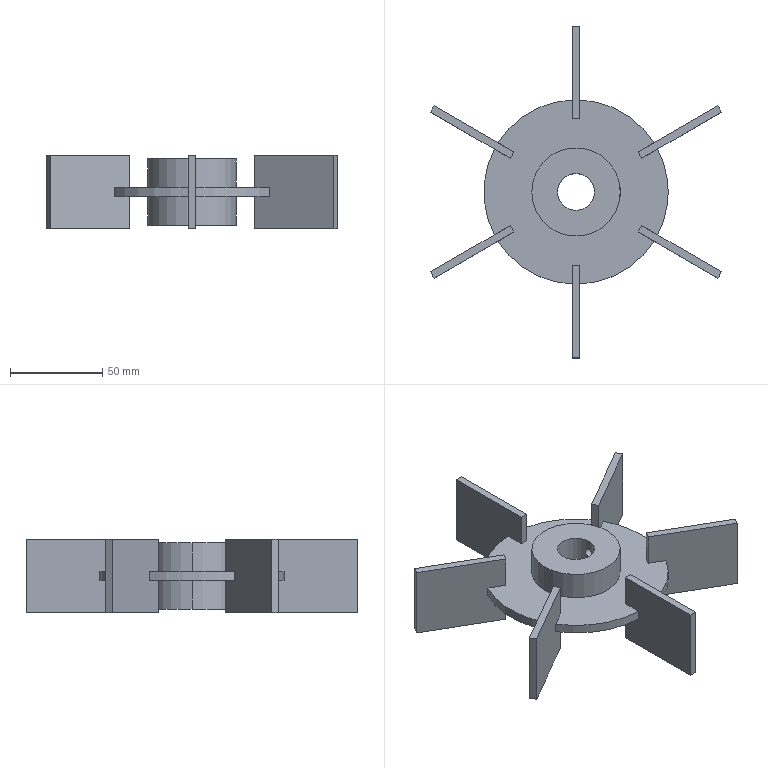Part | SolidWorks | features ICE 4, 3DProfileFeature 1, BaseBody 1, CirPattern 1, Cut 1, HoleWzd 1, Scale 1 | 1 solid | 63 faces | box 157.885 x 180 x 40 mm | volume 130306 mm3 | plane 46 | cylinder 17 | commonest cylinder face diameters 100 x7 5 x4 48 x4 20 x2